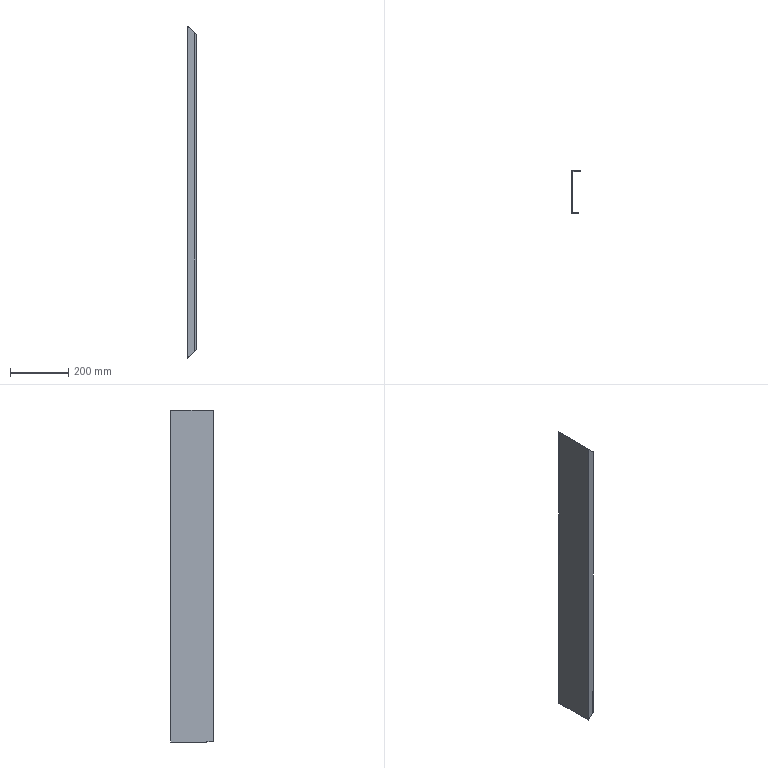Part | STEP file | 1519D1D1-4.stp.STEP | 1 solid | 12 faces | box 28 x 145 x 1139 mm | volume 261458 mm3 | plane 12
STEP:
#1=CARTESIAN_POINT('',(22.,1.2,-546.3));
#2=VERTEX_POINT('',#1);
#3=CARTESIAN_POINT('',(22.,1.2,547.5));
#4=VERTEX_POINT('',#3);
#5=CARTESIAN_POINT('',(22.,1.2,-546.3));
#6=DIRECTION('',(0.,0.,1.));
#7=VECTOR('',#6,1000.);
#8=LINE('',#5,#7);
#9=EDGE_CURVE('',#2,#4,#8,.T.);
#10=ORIENTED_EDGE('',*,*,#9,.T.);
#11=CARTESIAN_POINT('',(22.,0.,547.5));
#12=VERTEX_POINT('',#11);
#13=CARTESIAN_POINT('',(22.,0.,547.5));
#14=DIRECTION('',(0.,1.,0.));
#15=VECTOR('',#14,1000.);
#16=LINE('',#13,#15);
#17=EDGE_CURVE('',#12,#4,#16,.T.);
#18=ORIENTED_EDGE('',*,*,#17,.F.);
#19=CARTESIAN_POINT('',(22.,0.,-546.3));
#20=VERTEX_POINT('',#19);
#21=CARTESIAN_POINT('',(22.,0.,-546.3));
#22=DIRECTION('',(0.,0.,1.));
#23=VECTOR('',#22,1000.);
#24=LINE('',#21,#23);
#25=EDGE_CURVE('',#20,#12,#24,.T.);
#26=ORIENTED_EDGE('',*,*,#25,.F.);
#27=CARTESIAN_POINT('',(22.,0.,-546.3));
#28=DIRECTION('',(0.,1.,0.));
#29=VECTOR('',#28,1000.);
#30=LINE('',#27,#29);
#31=EDGE_CURVE('',#20,#2,#30,.T.);
#32=ORIENTED_EDGE('',*,*,#31,.T.);
#33=EDGE_LOOP('',(#10,#18,#26,#32));
#34=FACE_OUTER_BOUND('',#33,.T.);
#35=CARTESIAN_POINT('',(22.,0.,-569.5));
#36=DIRECTION('',(1.,0.,0.));
#37=DIRECTION('',(0.,1.,0.));
#38=AXIS2_PLACEMENT_3D('',#35,#36,#37);
#39=PLANE('',#38);
#40=ADVANCED_FACE('',(#34),#39,.T.);
#41=CARTESIAN_POINT('',(1.2,1.2,-567.1));
#42=VERTEX_POINT('',#41);
#43=CARTESIAN_POINT('',(1.2,21.2,-567.1));
#44=VERTEX_POINT('',#43);
#45=CARTESIAN_POINT('',(1.2,1.2,-567.1));
#46=DIRECTION('',(0.,1.,0.));
#47=VECTOR('',#46,1000.);
#48=LINE('',#45,#47);
#49=EDGE_CURVE('',#42,#44,#48,.T.);
#50=ORIENTED_EDGE('',*,*,#49,.F.);
#51=CARTESIAN_POINT('',(22.,1.2,-546.3));
#52=DIRECTION('',(-0.7071,0.,-0.7071));
#53=VECTOR('',#52,1000.);
#54=LINE('',#51,#53);
#55=EDGE_CURVE('',#2,#42,#54,.T.);
#56=ORIENTED_EDGE('',*,*,#55,.F.);
#57=ORIENTED_EDGE('',*,*,#31,.F.);
#58=CARTESIAN_POINT('',(0.,0.,-568.3));
#59=VERTEX_POINT('',#58);
#60=CARTESIAN_POINT('',(22.,0.,-546.3));
#61=DIRECTION('',(-0.7071,0.,-0.7071));
#62=VECTOR('',#61,1000.);
#63=LINE('',#60,#62);
#64=EDGE_CURVE('',#20,#59,#63,.T.);
#65=ORIENTED_EDGE('',*,*,#64,.T.);
#66=CARTESIAN_POINT('',(0.,21.2,-568.3));
#67=VERTEX_POINT('',#66);
#68=CARTESIAN_POINT('',(0.,0.,-568.3));
#69=DIRECTION('',(0.,1.,0.));
#70=VECTOR('',#69,1000.);
#71=LINE('',#68,#70);
#72=EDGE_CURVE('',#59,#67,#71,.T.);
#73=ORIENTED_EDGE('',*,*,#72,.T.);
#74=CARTESIAN_POINT('',(1.2,21.2,-567.1));
#75=DIRECTION('',(-0.7071,0.,-0.7071));
#76=VECTOR('',#75,1000.);
#77=LINE('',#74,#76);
#78=EDGE_CURVE('',#44,#67,#77,.T.);
#79=ORIENTED_EDGE('',*,*,#78,.F.);
#80=EDGE_LOOP('',(#50,#56,#57,#65,#73,#79));
#81=FACE_OUTER_BOUND('',#80,.T.);
#82=CARTESIAN_POINT('',(28.,0.,-540.3));
#83=DIRECTION('',(-0.7071,0.,0.7071));
#84=DIRECTION('',(0.,1.,0.));
#85=AXIS2_PLACEMENT_3D('',#82,#83,#84);
#86=PLANE('',#85);
#87=ADVANCED_FACE('',(#81),#86,.F.);
#88=CARTESIAN_POINT('',(1.2,21.2,-568.3));
#89=VERTEX_POINT('',#88);
#90=CARTESIAN_POINT('',(1.2,21.2,-568.3));
#91=DIRECTION('',(0.,0.,1.));
#92=VECTOR('',#91,1000.);
#93=LINE('',#90,#92);
#94=EDGE_CURVE('',#89,#44,#93,.T.);
#95=ORIENTED_EDGE('',*,*,#94,.T.);
#96=ORIENTED_EDGE('',*,*,#78,.T.);
#97=CARTESIAN_POINT('',(0.,21.2,-569.5));
#98=VERTEX_POINT('',#97);
#99=CARTESIAN_POINT('',(0.,21.2,-569.5));
#100=DIRECTION('',(0.,0.,1.));
#101=VECTOR('',#100,1000.);
#102=LINE('',#99,#101);
#103=EDGE_CURVE('',#98,#67,#102,.T.);
#104=ORIENTED_EDGE('',*,*,#103,.F.);
#105=CARTESIAN_POINT('',(1.2,21.2,-568.3));
#106=DIRECTION('',(-0.7071,0.,-0.7071));
#107=VECTOR('',#106,1000.);
#108=LINE('',#105,#107);
#109=EDGE_CURVE('',#89,#98,#108,.T.);
#110=ORIENTED_EDGE('',*,*,#109,.F.);
#111=EDGE_LOOP('',(#95,#96,#104,#110));
#112=FACE_OUTER_BOUND('',#111,.T.);
#113=CARTESIAN_POINT('',(0.,21.2,-569.5));
#114=DIRECTION('',(0.,-1.,0.));
#115=DIRECTION('',(0.,0.,-1.));
#116=AXIS2_PLACEMENT_3D('',#113,#114,#115);
#117=PLANE('',#116);
#118=ADVANCED_FACE('',(#112),#117,.T.);
#119=CARTESIAN_POINT('',(0.,145.,-569.5));
#120=VERTEX_POINT('',#119);
#121=CARTESIAN_POINT('',(0.,21.2,-569.5));
#122=DIRECTION('',(0.,1.,0.));
#123=VECTOR('',#122,1000.);
#124=LINE('',#121,#123);
#125=EDGE_CURVE('',#98,#120,#124,.T.);
#126=ORIENTED_EDGE('',*,*,#125,.T.);
#127=CARTESIAN_POINT('',(28.,145.,-541.5));
#128=VERTEX_POINT('',#127);
#129=CARTESIAN_POINT('',(28.,145.,-541.5));
#130=DIRECTION('',(-0.7071,0.,-0.7071));
#131=VECTOR('',#130,1000.);
#132=LINE('',#129,#131);
#133=EDGE_CURVE('',#128,#120,#132,.T.);
#134=ORIENTED_EDGE('',*,*,#133,.F.);
#135=CARTESIAN_POINT('',(28.,143.8,-541.5));
#136=VERTEX_POINT('',#135);
#137=CARTESIAN_POINT('',(28.,143.8,-541.5));
#138=DIRECTION('',(0.,1.,0.));
#139=VECTOR('',#138,1000.);
#140=LINE('',#137,#139);
#141=EDGE_CURVE('',#136,#128,#140,.T.);
#142=ORIENTED_EDGE('',*,*,#141,.F.);
#143=CARTESIAN_POINT('',(1.2,143.8,-568.3));
#144=VERTEX_POINT('',#143);
#145=CARTESIAN_POINT('',(28.,143.8,-541.5));
#146=DIRECTION('',(-0.7071,0.,-0.7071));
#147=VECTOR('',#146,1000.);
#148=LINE('',#145,#147);
#149=EDGE_CURVE('',#136,#144,#148,.T.);
#150=ORIENTED_EDGE('',*,*,#149,.T.);
#151=CARTESIAN_POINT('',(1.2,21.2,-568.3));
#152=DIRECTION('',(0.,1.,0.));
#153=VECTOR('',#152,1000.);
#154=LINE('',#151,#153);
#155=EDGE_CURVE('',#89,#144,#154,.T.);
#156=ORIENTED_EDGE('',*,*,#155,.F.);
#157=ORIENTED_EDGE('',*,*,#109,.T.);
#158=EDGE_LOOP('',(#126,#134,#142,#150,#156,#157));
#159=FACE_OUTER_BOUND('',#158,.T.);
#160=CARTESIAN_POINT('',(28.,0.,-541.5));
#161=DIRECTION('',(-0.7071,0.,0.7071));
#162=DIRECTION('',(0.,1.,0.));
#163=AXIS2_PLACEMENT_3D('',#160,#161,#162);
#164=PLANE('',#163);
#165=ADVANCED_FACE('',(#159),#164,.F.);
#166=ORIENTED_EDGE('',*,*,#155,.T.);
#167=CARTESIAN_POINT('',(1.2,143.8,568.3));
#168=VERTEX_POINT('',#167);
#169=CARTESIAN_POINT('',(1.2,143.8,-568.3));
#170=DIRECTION('',(0.,0.,1.));
#171=VECTOR('',#170,1000.);
#172=LINE('',#169,#171);
#173=EDGE_CURVE('',#144,#168,#172,.T.);
#174=ORIENTED_EDGE('',*,*,#173,.T.);
#175=CARTESIAN_POINT('',(1.2,1.2,568.3));
#176=VERTEX_POINT('',#175);
#177=CARTESIAN_POINT('',(1.2,1.2,568.3));
#178=DIRECTION('',(0.,1.,0.));
#179=VECTOR('',#178,1000.);
#180=LINE('',#177,#179);
#181=EDGE_CURVE('',#176,#168,#180,.T.);
#182=ORIENTED_EDGE('',*,*,#181,.F.);
#183=CARTESIAN_POINT('',(1.2,1.2,-567.1));
#184=DIRECTION('',(0.,0.,1.));
#185=VECTOR('',#184,1000.);
#186=LINE('',#183,#185);
#187=EDGE_CURVE('',#42,#176,#186,.T.);
#188=ORIENTED_EDGE('',*,*,#187,.F.);
#189=ORIENTED_EDGE('',*,*,#49,.T.);
#190=ORIENTED_EDGE('',*,*,#94,.F.);
#191=EDGE_LOOP('',(#166,#174,#182,#188,#189,#190));
#192=FACE_OUTER_BOUND('',#191,.T.);
#193=CARTESIAN_POINT('',(1.2,1.2,-569.5));
#194=DIRECTION('',(1.,0.,0.));
#195=DIRECTION('',(0.,1.,0.));
#196=AXIS2_PLACEMENT_3D('',#193,#194,#195);
#197=PLANE('',#196);
#198=ADVANCED_FACE('',(#192),#197,.T.);
#199=ORIENTED_EDGE('',*,*,#187,.T.);
#200=CARTESIAN_POINT('',(22.,1.2,547.5));
#201=DIRECTION('',(-0.7071,0.,0.7071));
#202=VECTOR('',#201,1000.);
#203=LINE('',#200,#202);
#204=EDGE_CURVE('',#4,#176,#203,.T.);
#205=ORIENTED_EDGE('',*,*,#204,.F.);
#206=ORIENTED_EDGE('',*,*,#9,.F.);
#207=ORIENTED_EDGE('',*,*,#55,.T.);
#208=EDGE_LOOP('',(#199,#205,#206,#207));
#209=FACE_OUTER_BOUND('',#208,.T.);
#210=CARTESIAN_POINT('',(22.,1.2,-569.5));
#211=DIRECTION('',(0.,1.,0.));
#212=DIRECTION('',(1.,0.,0.));
#213=AXIS2_PLACEMENT_3D('',#210,#211,#212);
#214=PLANE('',#213);
#215=ADVANCED_FACE('',(#209),#214,.T.);
#216=CARTESIAN_POINT('',(0.,0.,569.5));
#217=VERTEX_POINT('',#216);
#218=CARTESIAN_POINT('',(0.,145.,569.5));
#219=VERTEX_POINT('',#218);
#220=CARTESIAN_POINT('',(0.,0.,569.5));
#221=DIRECTION('',(0.,1.,0.));
#222=VECTOR('',#221,1000.);
#223=LINE('',#220,#222);
#224=EDGE_CURVE('',#217,#219,#223,.T.);
#225=ORIENTED_EDGE('',*,*,#224,.F.);
#226=CARTESIAN_POINT('',(22.,0.,547.5));
#227=DIRECTION('',(-0.7071,0.,0.7071));
#228=VECTOR('',#227,1000.);
#229=LINE('',#226,#228);
#230=EDGE_CURVE('',#12,#217,#229,.T.);
#231=ORIENTED_EDGE('',*,*,#230,.F.);
#232=ORIENTED_EDGE('',*,*,#17,.T.);
#233=ORIENTED_EDGE('',*,*,#204,.T.);
#234=ORIENTED_EDGE('',*,*,#181,.T.);
#235=CARTESIAN_POINT('',(28.,143.8,541.5));
#236=VERTEX_POINT('',#235);
#237=CARTESIAN_POINT('',(1.2,143.8,568.3));
#238=DIRECTION('',(0.7071,0.,-0.7071));
#239=VECTOR('',#238,1000.);
#240=LINE('',#237,#239);
#241=EDGE_CURVE('',#168,#236,#240,.T.);
#242=ORIENTED_EDGE('',*,*,#241,.T.);
#243=CARTESIAN_POINT('',(28.,145.,541.5));
#244=VERTEX_POINT('',#243);
#245=CARTESIAN_POINT('',(28.,143.8,541.5));
#246=DIRECTION('',(0.,1.,0.));
#247=VECTOR('',#246,1000.);
#248=LINE('',#245,#247);
#249=EDGE_CURVE('',#236,#244,#248,.T.);
#250=ORIENTED_EDGE('',*,*,#249,.T.);
#251=CARTESIAN_POINT('',(0.,145.,569.5));
#252=DIRECTION('',(0.7071,0.,-0.7071));
#253=VECTOR('',#252,1000.);
#254=LINE('',#251,#253);
#255=EDGE_CURVE('',#219,#244,#254,.T.);
#256=ORIENTED_EDGE('',*,*,#255,.F.);
#257=EDGE_LOOP('',(#225,#231,#232,#233,#234,#242,#250,#256));
#258=FACE_OUTER_BOUND('',#257,.T.);
#259=CARTESIAN_POINT('',(0.,0.,569.5));
#260=DIRECTION('',(-0.7071,0.,-0.7071));
#261=DIRECTION('',(-0.7071,0.,0.7071));
#262=AXIS2_PLACEMENT_3D('',#259,#260,#261);
#263=PLANE('',#262);
#264=ADVANCED_FACE('',(#258),#263,.F.);
#265=ORIENTED_EDGE('',*,*,#255,.T.);
#266=CARTESIAN_POINT('',(28.,145.,-541.5));
#267=DIRECTION('',(0.,0.,1.));
#268=VECTOR('',#267,1000.);
#269=LINE('',#266,#268);
#270=EDGE_CURVE('',#128,#244,#269,.T.);
#271=ORIENTED_EDGE('',*,*,#270,.F.);
#272=ORIENTED_EDGE('',*,*,#133,.T.);
#273=CARTESIAN_POINT('',(0.,145.,-569.5));
#274=DIRECTION('',(0.,0.,1.));
#275=VECTOR('',#274,1000.);
#276=LINE('',#273,#275);
#277=EDGE_CURVE('',#120,#219,#276,.T.);
#278=ORIENTED_EDGE('',*,*,#277,.T.);
#279=EDGE_LOOP('',(#265,#271,#272,#278));
#280=FACE_OUTER_BOUND('',#279,.T.);
#281=CARTESIAN_POINT('',(28.,145.,-569.5));
#282=DIRECTION('',(0.,1.,0.));
#283=DIRECTION('',(1.,0.,0.));
#284=AXIS2_PLACEMENT_3D('',#281,#282,#283);
#285=PLANE('',#284);
#286=ADVANCED_FACE('',(#280),#285,.T.);
#287=ORIENTED_EDGE('',*,*,#72,.F.);
#288=CARTESIAN_POINT('',(0.,0.,-568.3));
#289=DIRECTION('',(0.,0.,1.));
#290=VECTOR('',#289,1000.);
#291=LINE('',#288,#290);
#292=EDGE_CURVE('',#59,#217,#291,.T.);
#293=ORIENTED_EDGE('',*,*,#292,.T.);
#294=ORIENTED_EDGE('',*,*,#224,.T.);
#295=ORIENTED_EDGE('',*,*,#277,.F.);
#296=ORIENTED_EDGE('',*,*,#125,.F.);
#297=ORIENTED_EDGE('',*,*,#103,.T.);
#298=EDGE_LOOP('',(#287,#293,#294,#295,#296,#297));
#299=FACE_OUTER_BOUND('',#298,.T.);
#300=CARTESIAN_POINT('',(0.,145.,-569.5));
#301=DIRECTION('',(-1.,0.,0.));
#302=DIRECTION('',(0.,0.,1.));
#303=AXIS2_PLACEMENT_3D('',#300,#301,#302);
#304=PLANE('',#303);
#305=ADVANCED_FACE('',(#299),#304,.T.);
#306=ORIENTED_EDGE('',*,*,#64,.F.);
#307=ORIENTED_EDGE('',*,*,#25,.T.);
#308=ORIENTED_EDGE('',*,*,#230,.T.);
#309=ORIENTED_EDGE('',*,*,#292,.F.);
#310=EDGE_LOOP('',(#306,#307,#308,#309));
#311=FACE_OUTER_BOUND('',#310,.T.);
#312=CARTESIAN_POINT('',(0.,0.,-569.5));
#313=DIRECTION('',(0.,-1.,0.));
#314=DIRECTION('',(0.,0.,-1.));
#315=AXIS2_PLACEMENT_3D('',#312,#313,#314);
#316=PLANE('',#315);
#317=ADVANCED_FACE('',(#311),#316,.T.);
#318=CARTESIAN_POINT('',(28.,143.8,-541.5));
#319=DIRECTION('',(0.,0.,1.));
#320=VECTOR('',#319,1000.);
#321=LINE('',#318,#320);
#322=EDGE_CURVE('',#136,#236,#321,.T.);
#323=ORIENTED_EDGE('',*,*,#322,.F.);
#324=ORIENTED_EDGE('',*,*,#141,.T.);
#325=ORIENTED_EDGE('',*,*,#270,.T.);
#326=ORIENTED_EDGE('',*,*,#249,.F.);
#327=EDGE_LOOP('',(#323,#324,#325,#326));
#328=FACE_OUTER_BOUND('',#327,.T.);
#329=CARTESIAN_POINT('',(28.,143.8,-569.5));
#330=DIRECTION('',(1.,0.,0.));
#331=DIRECTION('',(0.,1.,0.));
#332=AXIS2_PLACEMENT_3D('',#329,#330,#331);
#333=PLANE('',#332);
#334=ADVANCED_FACE('',(#328),#333,.T.);
#335=ORIENTED_EDGE('',*,*,#173,.F.);
#336=ORIENTED_EDGE('',*,*,#149,.F.);
#337=ORIENTED_EDGE('',*,*,#322,.T.);
#338=ORIENTED_EDGE('',*,*,#241,.F.);
#339=EDGE_LOOP('',(#335,#336,#337,#338));
#340=FACE_OUTER_BOUND('',#339,.T.);
#341=CARTESIAN_POINT('',(1.2,143.8,-569.5));
#342=DIRECTION('',(0.,-1.,0.));
#343=DIRECTION('',(0.,0.,-1.));
#344=AXIS2_PLACEMENT_3D('',#341,#342,#343);
#345=PLANE('',#344);
#346=ADVANCED_FACE('',(#340),#345,.T.);
#347=CLOSED_SHELL('',(#40,#87,#118,#165,#198,#215,#264,#286,#305,#317,#334,#346));
#348=MANIFOLD_SOLID_BREP('',#347);
#349=CARTESIAN_POINT('',(0.,0.,0.));
#350=DIRECTION('',(0.,0.,1.));
#351=DIRECTION('',(1.,0.,0.));
#352=AXIS2_PLACEMENT_3D('',#349,#350,#351);
#353=(LENGTH_UNIT()NAMED_UNIT(*)SI_UNIT(.MILLI.,.METRE.));
#354=UNCERTAINTY_MEASURE_WITH_UNIT(LENGTH_MEASURE(0.00001),#353,'','');
#355=(NAMED_UNIT(*)PLANE_ANGLE_UNIT()SI_UNIT($,.RADIAN.));
#356=(NAMED_UNIT(*)SI_UNIT($,.STERADIAN.)SOLID_ANGLE_UNIT());
#357=(GEOMETRIC_REPRESENTATION_CONTEXT(3)GLOBAL_UNCERTAINTY_ASSIGNED_CONTEXT((#354))GLOBAL_UNIT_ASSIGNED_CONTEXT((#353,#355,#356))REPRESENTATION_CONTEXT('',''));
#358=ADVANCED_BREP_SHAPE_REPRESENTATION('',(#348,#352),#357);